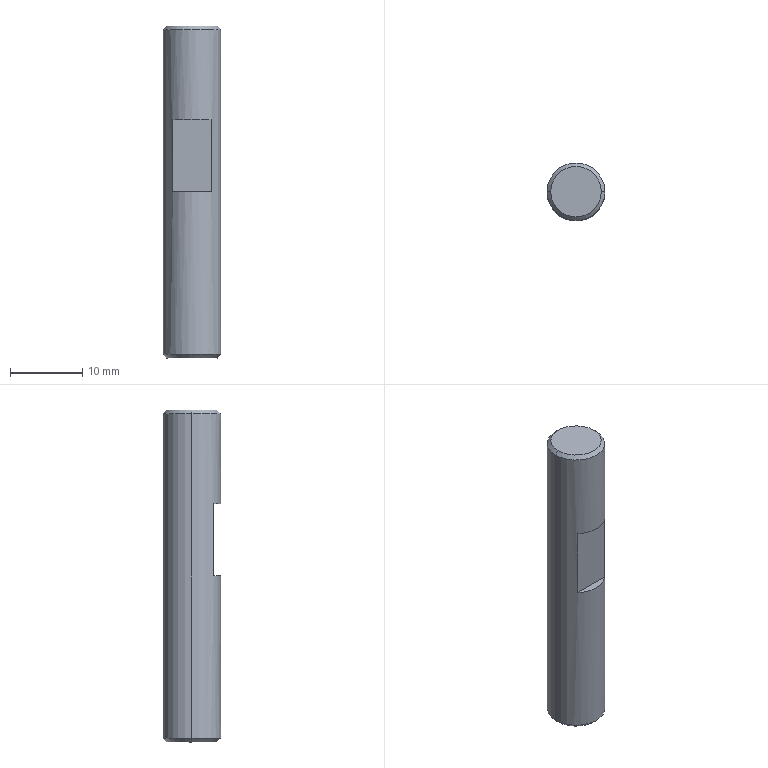Part | NX | 1 solid | 11 faces | box 8 x 8 x 46 mm | volume 2270 mm3 | plane 5 | cone 4 | cylinder 2 | commonest cylinder face diameters 8 x2
STEP:
#1=CARTESIAN_POINT('',(-3.5,0.,0.));
#2=VERTEX_POINT('',#1);
#3=CARTESIAN_POINT('',(3.5,0.,0.));
#4=VERTEX_POINT('',#3);
#5=CARTESIAN_POINT('',(0.,0.,0.));
#6=DIRECTION('',(0.,0.,1.));
#7=DIRECTION('',(-1.,0.,0.));
#8=AXIS2_PLACEMENT_3D('',#5,#6,#7);
#9=CIRCLE('',#8,3.5);
#10=EDGE_CURVE('',#2,#4,#9,.T.);
#11=ORIENTED_EDGE('',*,*,#10,.F.);
#12=CARTESIAN_POINT('',(0.,0.,0.));
#13=DIRECTION('',(0.,0.,1.));
#14=DIRECTION('',(-1.,0.,0.));
#15=AXIS2_PLACEMENT_3D('',#12,#13,#14);
#16=CIRCLE('',#15,3.5);
#17=EDGE_CURVE('',#4,#2,#16,.T.);
#18=ORIENTED_EDGE('',*,*,#17,.F.);
#19=EDGE_LOOP('',(#11,#18));
#20=FACE_BOUND('',#19,.T.);
#21=CARTESIAN_POINT('',(0.,0.,0.));
#22=DIRECTION('',(0.,0.,1.));
#23=DIRECTION('',(1.,0.,0.));
#24=AXIS2_PLACEMENT_3D('',#21,#22,#23);
#25=PLANE('',#24);
#26=ADVANCED_FACE('',(#20),#25,.F.);
#27=CARTESIAN_POINT('',(4.,0.,0.5));
#28=VERTEX_POINT('',#27);
#29=CARTESIAN_POINT('',(-4.,0.,0.5));
#30=VERTEX_POINT('',#29);
#31=CARTESIAN_POINT('',(0.,0.,0.5));
#32=DIRECTION('',(0.,0.,1.));
#33=DIRECTION('',(-1.,0.,0.));
#34=AXIS2_PLACEMENT_3D('',#31,#32,#33);
#35=CIRCLE('',#34,4.);
#36=EDGE_CURVE('',#28,#30,#35,.T.);
#37=ORIENTED_EDGE('',*,*,#36,.F.);
#38=CARTESIAN_POINT('',(3.75,0.,0.25));
#39=DIRECTION('',(0.7071,0.,0.7071));
#40=VECTOR('',#39,1000.);
#41=LINE('',#38,#40);
#42=EDGE_CURVE('',#4,#28,#41,.T.);
#43=ORIENTED_EDGE('',*,*,#42,.F.);
#44=ORIENTED_EDGE('',*,*,#17,.T.);
#45=CARTESIAN_POINT('',(-3.75,0.,0.25));
#46=DIRECTION('',(-0.7071,0.,0.7071));
#47=VECTOR('',#46,1000.);
#48=LINE('',#45,#47);
#49=EDGE_CURVE('',#2,#30,#48,.T.);
#50=ORIENTED_EDGE('',*,*,#49,.T.);
#51=EDGE_LOOP('',(#37,#43,#44,#50));
#52=FACE_BOUND('',#51,.T.);
#53=CARTESIAN_POINT('',(0.,0.,0.25));
#54=DIRECTION('',(0.,0.,1.));
#55=DIRECTION('',(1.,0.,0.));
#56=AXIS2_PLACEMENT_3D('',#53,#54,#55);
#57=CONICAL_SURFACE('',#56,3.75,0.7854);
#58=ADVANCED_FACE('',(#52),#57,.T.);
#59=CARTESIAN_POINT('',(-2.646,-3.,33.));
#60=VERTEX_POINT('',#59);
#61=CARTESIAN_POINT('',(2.646,-3.,33.));
#62=VERTEX_POINT('',#61);
#63=CARTESIAN_POINT('',(0.,0.,33.));
#64=DIRECTION('',(0.,0.,1.));
#65=DIRECTION('',(-0.6614,-0.75,0.));
#66=AXIS2_PLACEMENT_3D('',#63,#64,#65);
#67=CIRCLE('',#66,4.);
#68=EDGE_CURVE('',#60,#62,#67,.T.);
#69=ORIENTED_EDGE('',*,*,#68,.F.);
#70=CARTESIAN_POINT('',(2.646,-3.,33.));
#71=DIRECTION('',(-1.,0.,0.));
#72=VECTOR('',#71,1000.);
#73=LINE('',#70,#72);
#74=EDGE_CURVE('',#62,#60,#73,.T.);
#75=ORIENTED_EDGE('',*,*,#74,.F.);
#76=EDGE_LOOP('',(#69,#75));
#77=FACE_BOUND('',#76,.T.);
#78=CARTESIAN_POINT('',(-4.8,-4.,33.));
#79=DIRECTION('',(0.,0.,1.));
#80=DIRECTION('',(1.,0.,0.));
#81=AXIS2_PLACEMENT_3D('',#78,#79,#80);
#82=PLANE('',#81);
#83=ADVANCED_FACE('',(#77),#82,.F.);
#84=ORIENTED_EDGE('',*,*,#36,.T.);
#85=CARTESIAN_POINT('',(-4.,0.,45.5));
#86=VERTEX_POINT('',#85);
#87=CARTESIAN_POINT('',(-4.,0.,0.));
#88=DIRECTION('',(0.,0.,1.));
#89=VECTOR('',#88,1000.);
#90=LINE('',#87,#89);
#91=EDGE_CURVE('',#86,#30,#90,.F.);
#92=ORIENTED_EDGE('',*,*,#91,.F.);
#93=CARTESIAN_POINT('',(4.,0.,45.5));
#94=VERTEX_POINT('',#93);
#95=CARTESIAN_POINT('',(0.,0.,45.5));
#96=DIRECTION('',(0.,0.,-1.));
#97=DIRECTION('',(1.,0.,0.));
#98=AXIS2_PLACEMENT_3D('',#95,#96,#97);
#99=CIRCLE('',#98,4.);
#100=EDGE_CURVE('',#86,#94,#99,.T.);
#101=ORIENTED_EDGE('',*,*,#100,.T.);
#102=CARTESIAN_POINT('',(4.,0.,0.));
#103=DIRECTION('',(0.,0.,1.));
#104=VECTOR('',#103,1000.);
#105=LINE('',#102,#104);
#106=EDGE_CURVE('',#94,#28,#105,.F.);
#107=ORIENTED_EDGE('',*,*,#106,.T.);
#108=EDGE_LOOP('',(#84,#92,#101,#107));
#109=FACE_BOUND('',#108,.T.);
#110=CARTESIAN_POINT('',(0.,0.,0.));
#111=DIRECTION('',(0.,0.,1.));
#112=DIRECTION('',(1.,0.,0.));
#113=AXIS2_PLACEMENT_3D('',#110,#111,#112);
#114=CYLINDRICAL_SURFACE('',#113,4.);
#115=ADVANCED_FACE('',(#109),#114,.T.);
#116=CARTESIAN_POINT('',(2.646,-3.,23.));
#117=VERTEX_POINT('',#116);
#118=CARTESIAN_POINT('',(-2.646,-3.,23.));
#119=VERTEX_POINT('',#118);
#120=CARTESIAN_POINT('',(0.,0.,23.));
#121=DIRECTION('',(0.,0.,-1.));
#122=DIRECTION('',(0.6614,-0.75,0.));
#123=AXIS2_PLACEMENT_3D('',#120,#121,#122);
#124=CIRCLE('',#123,4.);
#125=EDGE_CURVE('',#117,#119,#124,.T.);
#126=ORIENTED_EDGE('',*,*,#125,.F.);
#127=CARTESIAN_POINT('',(2.646,-3.,23.));
#128=DIRECTION('',(-1.,0.,0.));
#129=VECTOR('',#128,1000.);
#130=LINE('',#127,#129);
#131=EDGE_CURVE('',#117,#119,#130,.T.);
#132=ORIENTED_EDGE('',*,*,#131,.T.);
#133=EDGE_LOOP('',(#126,#132));
#134=FACE_BOUND('',#133,.T.);
#135=CARTESIAN_POINT('',(-4.8,-3.,23.));
#136=DIRECTION('',(0.,0.,-1.));
#137=DIRECTION('',(0.,-1.,0.));
#138=AXIS2_PLACEMENT_3D('',#135,#136,#137);
#139=PLANE('',#138);
#140=ADVANCED_FACE('',(#134),#139,.F.);
#141=CARTESIAN_POINT('',(0.,0.,45.5));
#142=DIRECTION('',(0.,0.,-1.));
#143=DIRECTION('',(1.,0.,0.));
#144=AXIS2_PLACEMENT_3D('',#141,#142,#143);
#145=CIRCLE('',#144,4.);
#146=EDGE_CURVE('',#94,#86,#145,.T.);
#147=ORIENTED_EDGE('',*,*,#146,.F.);
#148=CARTESIAN_POINT('',(3.5,0.,46.));
#149=VERTEX_POINT('',#148);
#150=CARTESIAN_POINT('',(3.75,0.,45.75));
#151=DIRECTION('',(0.7071,0.,-0.7071));
#152=VECTOR('',#151,1000.);
#153=LINE('',#150,#152);
#154=EDGE_CURVE('',#149,#94,#153,.T.);
#155=ORIENTED_EDGE('',*,*,#154,.F.);
#156=CARTESIAN_POINT('',(-3.5,0.,46.));
#157=VERTEX_POINT('',#156);
#158=CARTESIAN_POINT('',(0.,0.,46.));
#159=DIRECTION('',(0.,0.,-1.));
#160=DIRECTION('',(1.,0.,0.));
#161=AXIS2_PLACEMENT_3D('',#158,#159,#160);
#162=CIRCLE('',#161,3.5);
#163=EDGE_CURVE('',#149,#157,#162,.T.);
#164=ORIENTED_EDGE('',*,*,#163,.T.);
#165=CARTESIAN_POINT('',(-3.75,0.,45.75));
#166=DIRECTION('',(-0.7071,0.,-0.7071));
#167=VECTOR('',#166,1000.);
#168=LINE('',#165,#167);
#169=EDGE_CURVE('',#157,#86,#168,.T.);
#170=ORIENTED_EDGE('',*,*,#169,.T.);
#171=EDGE_LOOP('',(#147,#155,#164,#170));
#172=FACE_BOUND('',#171,.T.);
#173=CARTESIAN_POINT('',(0.,0.,45.75));
#174=DIRECTION('',(0.,0.,-1.));
#175=DIRECTION('',(-1.,0.,0.));
#176=AXIS2_PLACEMENT_3D('',#173,#174,#175);
#177=CONICAL_SURFACE('',#176,3.75,0.7854);
#178=ADVANCED_FACE('',(#172),#177,.T.);
#179=CARTESIAN_POINT('',(0.,0.,46.));
#180=DIRECTION('',(0.,0.,-1.));
#181=DIRECTION('',(1.,0.,0.));
#182=AXIS2_PLACEMENT_3D('',#179,#180,#181);
#183=CIRCLE('',#182,3.5);
#184=EDGE_CURVE('',#157,#149,#183,.T.);
#185=ORIENTED_EDGE('',*,*,#184,.F.);
#186=ORIENTED_EDGE('',*,*,#163,.F.);
#187=EDGE_LOOP('',(#185,#186));
#188=FACE_BOUND('',#187,.T.);
#189=CARTESIAN_POINT('',(0.,0.,46.));
#190=DIRECTION('',(0.,0.,1.));
#191=DIRECTION('',(1.,0.,0.));
#192=AXIS2_PLACEMENT_3D('',#189,#190,#191);
#193=PLANE('',#192);
#194=ADVANCED_FACE('',(#188),#193,.T.);
#195=CARTESIAN_POINT('',(-2.646,-3.,33.));
#196=DIRECTION('',(0.,0.,-1.));
#197=VECTOR('',#196,1000.);
#198=LINE('',#195,#197);
#199=EDGE_CURVE('',#60,#119,#198,.T.);
#200=ORIENTED_EDGE('',*,*,#199,.T.);
#201=ORIENTED_EDGE('',*,*,#131,.F.);
#202=CARTESIAN_POINT('',(2.646,-3.,23.));
#203=DIRECTION('',(0.,0.,1.));
#204=VECTOR('',#203,1000.);
#205=LINE('',#202,#204);
#206=EDGE_CURVE('',#117,#62,#205,.T.);
#207=ORIENTED_EDGE('',*,*,#206,.T.);
#208=ORIENTED_EDGE('',*,*,#74,.T.);
#209=EDGE_LOOP('',(#200,#201,#207,#208));
#210=FACE_BOUND('',#209,.T.);
#211=CARTESIAN_POINT('',(-4.8,-3.,33.));
#212=DIRECTION('',(0.,1.,0.));
#213=DIRECTION('',(1.,0.,0.));
#214=AXIS2_PLACEMENT_3D('',#211,#212,#213);
#215=PLANE('',#214);
#216=ADVANCED_FACE('',(#210),#215,.F.);
#217=ORIENTED_EDGE('',*,*,#146,.T.);
#218=ORIENTED_EDGE('',*,*,#91,.T.);
#219=CARTESIAN_POINT('',(0.,0.,0.5));
#220=DIRECTION('',(0.,0.,1.));
#221=DIRECTION('',(-1.,0.,0.));
#222=AXIS2_PLACEMENT_3D('',#219,#220,#221);
#223=CIRCLE('',#222,4.);
#224=EDGE_CURVE('',#30,#28,#223,.T.);
#225=ORIENTED_EDGE('',*,*,#224,.T.);
#226=ORIENTED_EDGE('',*,*,#106,.F.);
#227=EDGE_LOOP('',(#217,#218,#225,#226));
#228=FACE_BOUND('',#227,.T.);
#229=ORIENTED_EDGE('',*,*,#68,.T.);
#230=ORIENTED_EDGE('',*,*,#206,.F.);
#231=ORIENTED_EDGE('',*,*,#125,.T.);
#232=ORIENTED_EDGE('',*,*,#199,.F.);
#233=EDGE_LOOP('',(#229,#230,#231,#232));
#234=FACE_BOUND('',#233,.T.);
#235=CARTESIAN_POINT('',(0.,0.,0.));
#236=DIRECTION('',(0.,0.,1.));
#237=DIRECTION('',(1.,0.,0.));
#238=AXIS2_PLACEMENT_3D('',#235,#236,#237);
#239=CYLINDRICAL_SURFACE('',#238,4.);
#240=ADVANCED_FACE('',(#228,#234),#239,.T.);
#241=ORIENTED_EDGE('',*,*,#10,.T.);
#242=ORIENTED_EDGE('',*,*,#42,.T.);
#243=ORIENTED_EDGE('',*,*,#224,.F.);
#244=ORIENTED_EDGE('',*,*,#49,.F.);
#245=EDGE_LOOP('',(#241,#242,#243,#244));
#246=FACE_BOUND('',#245,.T.);
#247=CARTESIAN_POINT('',(0.,0.,0.25));
#248=DIRECTION('',(0.,0.,1.));
#249=DIRECTION('',(1.,0.,0.));
#250=AXIS2_PLACEMENT_3D('',#247,#248,#249);
#251=CONICAL_SURFACE('',#250,3.75,0.7854);
#252=ADVANCED_FACE('',(#246),#251,.T.);
#253=ORIENTED_EDGE('',*,*,#184,.T.);
#254=ORIENTED_EDGE('',*,*,#154,.T.);
#255=ORIENTED_EDGE('',*,*,#100,.F.);
#256=ORIENTED_EDGE('',*,*,#169,.F.);
#257=EDGE_LOOP('',(#253,#254,#255,#256));
#258=FACE_BOUND('',#257,.T.);
#259=CARTESIAN_POINT('',(0.,0.,45.75));
#260=DIRECTION('',(0.,0.,-1.));
#261=DIRECTION('',(-1.,0.,0.));
#262=AXIS2_PLACEMENT_3D('',#259,#260,#261);
#263=CONICAL_SURFACE('',#262,3.75,0.7854);
#264=ADVANCED_FACE('',(#258),#263,.T.);
#265=CLOSED_SHELL('',(#26,#58,#83,#115,#140,#178,#194,#216,#240,#252,#264));
#266=MANIFOLD_SOLID_BREP('',#265);
#267=(LENGTH_UNIT()NAMED_UNIT(*)SI_UNIT(.MILLI.,.METRE.));
#268=UNCERTAINTY_MEASURE_WITH_UNIT(LENGTH_MEASURE(0.00001),#267,'','');
#269=(NAMED_UNIT(*)PLANE_ANGLE_UNIT()SI_UNIT($,.RADIAN.));
#270=(NAMED_UNIT(*)SI_UNIT($,.STERADIAN.)SOLID_ANGLE_UNIT());
#271=(GEOMETRIC_REPRESENTATION_CONTEXT(3)GLOBAL_UNCERTAINTY_ASSIGNED_CONTEXT((#268))GLOBAL_UNIT_ASSIGNED_CONTEXT((#267,#269,#270))REPRESENTATION_CONTEXT('',''));
#272=ADVANCED_BREP_SHAPE_REPRESENTATION('',(#266),#271);